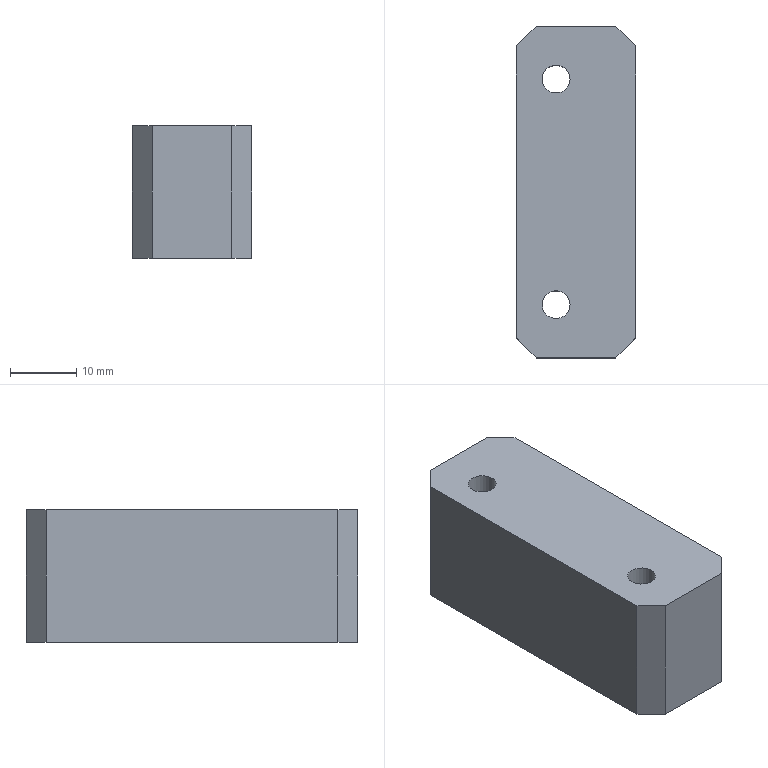CAM job | NX | 3-axis milling, drilling | part box 18 x 50 x 20 mm | stock box 20 x 55 x 25 mm
Tools:
number,name,description,diameter,corner_radius,flute_length,length,flutes
9,D10,平底铣刀-粗,10.0,0.0,35.0,75.0,2
10,D10-J,平底铣刀-精,10.0,0.0,35.0,75.0,2
1,D80R0.8飞刀,圆鼻刀-粗,80.0,0.8,50.0,75.0,2
2,D6倒角刀,倒角刀,6.0,0.0,3.0,25.0,2
22,M5X0.8,丝锥,4.2,0.0,35.0,50.0,2
14,钻头4.2,Twist Drill 4.2 mm,4.2,0.0,41.0,41.738,2
Operations:
program,operation,operation_type,tool,method,geometry_group,spindle_rpm,surface_speed,feed_per_tooth,feed_cut,feed_plunge,cut_length_mm,path_length_mm,cut_time_min,machine_time_min
A,顶面,FaceMilling,D80R0.8飞刀,侧刃精光-切深K-步距G,W-A,4000.0,1005.31,0.125,1000.0,100.0,144.0,180.0,0.144,0.1476
A,外形粗_2,VolumeBased25DMillingOperation,D10,METHOD,W-A,8000.0,251.327,0.3125,5000.0,80.0,4509.965,4568.965,0.902,0.9079
A,打点-深0.8,Operation,D6倒角刀,NONE,W-A,8000.0,150.796,0.0312,500.0,90.0,3.6,82.215,0.0072,0.0151
A,通孔-M5螺纹底孔,Operation,钻头4.2,NONE,W-A,3000.0,39.584,0.0583,350.0,90.0,56.524,188.062,0.1615,0.1746
A,仅选体,SurfaceContour,D6倒角刀,METHOD,W-A,8000.0,150.796,0.1875,3000.0,100.0,146.272,182.073,0.0488,0.0523
A,铣倒角_1,PlanarMilling,D6倒角刀,METHOD,W-A,8000.0,150.796,0.0312,500.0,100.0,36.041,153.428,0.0721,0.0838
A,通孔-攻牙M5,Operation,M5X0.8,METHOD,W-A,500.0,6.597,0.0008,0.8,90.0,49.0,173.015,61.25,61.262
A,外形半精_2,VolumeBased25DMillingOperation,D10-J,METHOD,W-A,8000.0,251.327,0.0625,1000.0,100.0,330.689,472.704,0.3307,0.3449